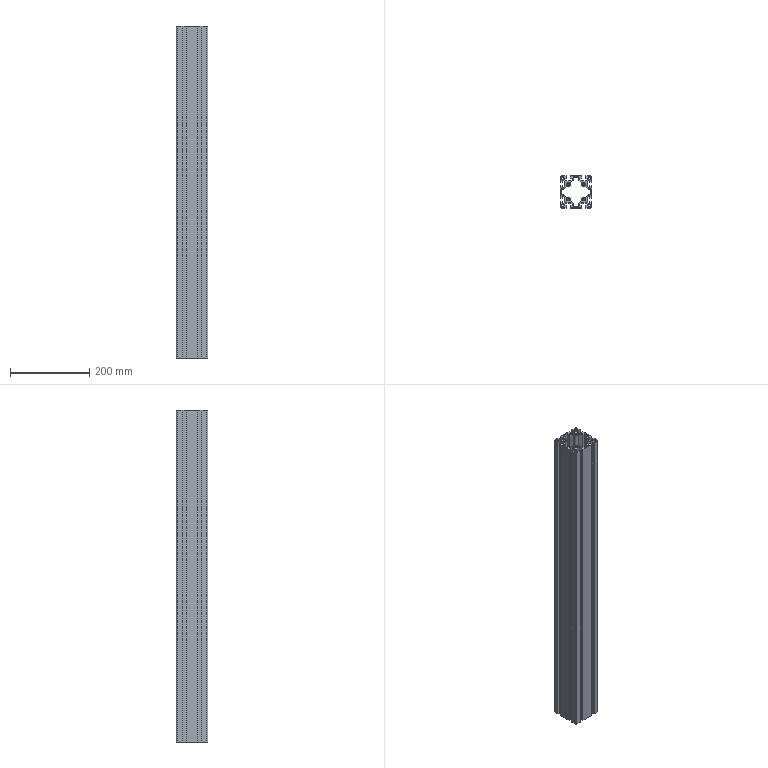Part | NX | 1 solid | 156 faces | box 80 x 80 x 840 mm | volume 1471682 mm3 | plane 122 | cylinder 34 | commonest cylinder face diameters 2 x16 6.8 x8 11.8 x6 5.64 x4